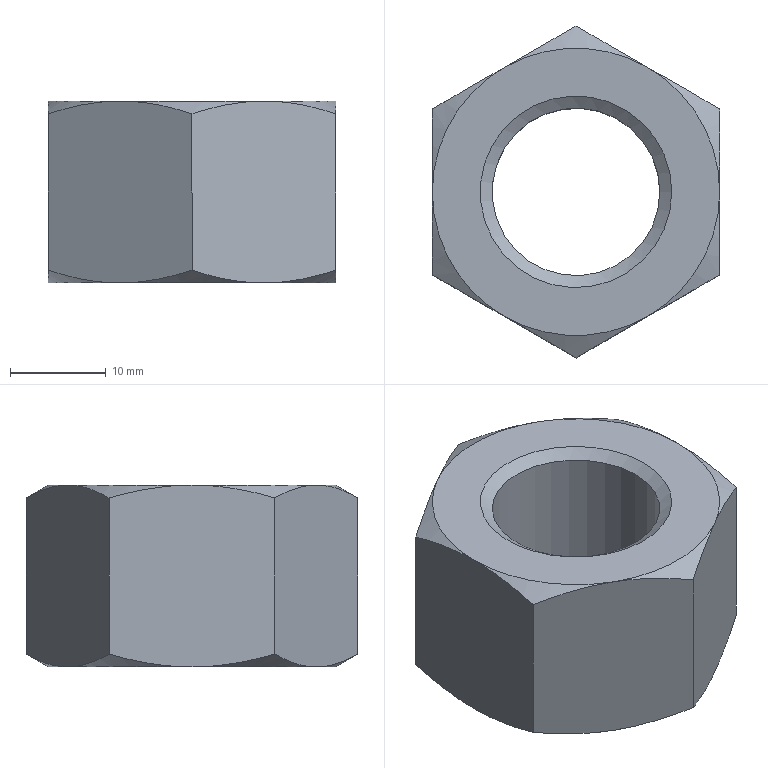Part | NX | features Hexagon Nut ISO - 4034 - M20 - N_Hexagon Nut ISO - 4034 - M20 - N 2 | 1 solid | 24 faces | box 30 x 34.641 x 19 mm | volume 10115 mm3 | cone 14 | plane 8 | cylinder 2 | commonest cylinder face diameters 17.5 x1 20 x1
STEP:
#1=CARTESIAN_POINT('',(7.5,12.99,-19.));
#2=VERTEX_POINT('',#1);
#3=CARTESIAN_POINT('',(15.,8.66,-17.66));
#4=VERTEX_POINT('',#3);
#5=CARTESIAN_POINT('',(7.5,12.99,-19.));
#6=CARTESIAN_POINT('',(10.06,11.512,-19.));
#7=CARTESIAN_POINT('',(12.55,10.075,-18.477));
#8=CARTESIAN_POINT('',(15.,8.66,-17.66));
#9=B_SPLINE_CURVE_WITH_KNOTS('',3,(#5,#6,#7,#8),.UNSPECIFIED.,.F.,.F.,(4,4),(0.,0.008763),.UNSPECIFIED.);
#10=EDGE_CURVE('',#2,#4,#9,.T.);
#11=ORIENTED_EDGE('',*,*,#10,.F.);
#12=CARTESIAN_POINT('',(-0.000000038,17.321,-17.66));
#13=VERTEX_POINT('',#12);
#14=CARTESIAN_POINT('',(-0.000000042,17.321,-17.66));
#15=CARTESIAN_POINT('',(2.45,15.906,-18.477));
#16=CARTESIAN_POINT('',(4.94,14.468,-19.));
#17=CARTESIAN_POINT('',(7.5,12.99,-19.));
#18=B_SPLINE_CURVE_WITH_KNOTS('',3,(#14,#15,#16,#17),.UNSPECIFIED.,.F.,.F.,(4,4),(0.,0.008763),.UNSPECIFIED.);
#19=EDGE_CURVE('',#13,#2,#18,.T.);
#20=ORIENTED_EDGE('',*,*,#19,.F.);
#21=CARTESIAN_POINT('',(0.000000038,17.321,-1.34));
#22=VERTEX_POINT('',#21);
#23=CARTESIAN_POINT('',(0.,17.321,-19.));
#24=DIRECTION('',(0.,0.,1.));
#25=VECTOR('',#24,1000.);
#26=LINE('',#23,#25);
#27=EDGE_CURVE('',#22,#13,#26,.F.);
#28=ORIENTED_EDGE('',*,*,#27,.F.);
#29=CARTESIAN_POINT('',(7.5,12.99,0.));
#30=VERTEX_POINT('',#29);
#31=CARTESIAN_POINT('',(7.5,12.99,0.));
#32=CARTESIAN_POINT('',(4.94,14.468,0.));
#33=CARTESIAN_POINT('',(2.45,15.906,-0.5229));
#34=CARTESIAN_POINT('',(0.000000075,17.321,-1.34));
#35=B_SPLINE_CURVE_WITH_KNOTS('',3,(#31,#32,#33,#34),.UNSPECIFIED.,.F.,.F.,(4,4),(0.,0.008763),.UNSPECIFIED.);
#36=EDGE_CURVE('',#30,#22,#35,.T.);
#37=ORIENTED_EDGE('',*,*,#36,.F.);
#38=CARTESIAN_POINT('',(15.,8.66,-1.34));
#39=VERTEX_POINT('',#38);
#40=CARTESIAN_POINT('',(15.,8.66,-1.34));
#41=CARTESIAN_POINT('',(12.55,10.075,-0.5229));
#42=CARTESIAN_POINT('',(10.06,11.512,0.));
#43=CARTESIAN_POINT('',(7.5,12.99,0.));
#44=B_SPLINE_CURVE_WITH_KNOTS('',3,(#40,#41,#42,#43),.UNSPECIFIED.,.F.,.F.,(4,4),(0.,0.008763),.UNSPECIFIED.);
#45=EDGE_CURVE('',#39,#30,#44,.T.);
#46=ORIENTED_EDGE('',*,*,#45,.F.);
#47=CARTESIAN_POINT('',(15.,8.66,-19.));
#48=DIRECTION('',(0.,0.,1.));
#49=VECTOR('',#48,1000.);
#50=LINE('',#47,#49);
#51=EDGE_CURVE('',#39,#4,#50,.F.);
#52=ORIENTED_EDGE('',*,*,#51,.T.);
#53=EDGE_LOOP('',(#11,#20,#28,#37,#46,#52));
#54=FACE_BOUND('',#53,.T.);
#55=CARTESIAN_POINT('',(15.,8.66,-19.));
#56=DIRECTION('',(0.5,0.866,0.));
#57=DIRECTION('',(-0.866,0.5,0.));
#58=AXIS2_PLACEMENT_3D('',#55,#56,#57);
#59=PLANE('',#58);
#60=ADVANCED_FACE('',(#54),#59,.T.);
#61=CARTESIAN_POINT('',(15.,-8.66,-17.66));
#62=VERTEX_POINT('',#61);
#63=CARTESIAN_POINT('',(15.,-8.66,-1.34));
#64=VERTEX_POINT('',#63);
#65=CARTESIAN_POINT('',(15.,-8.66,-19.));
#66=DIRECTION('',(0.,0.,1.));
#67=VECTOR('',#66,1000.);
#68=LINE('',#65,#67);
#69=EDGE_CURVE('',#62,#64,#68,.T.);
#70=ORIENTED_EDGE('',*,*,#69,.F.);
#71=CARTESIAN_POINT('',(15.,0.,-19.));
#72=VERTEX_POINT('',#71);
#73=CARTESIAN_POINT('',(15.,0.,-19.));
#74=CARTESIAN_POINT('',(15.,-2.956,-19.));
#75=CARTESIAN_POINT('',(15.,-5.831,-18.477));
#76=CARTESIAN_POINT('',(15.,-8.66,-17.66));
#77=B_SPLINE_CURVE_WITH_KNOTS('',3,(#73,#74,#75,#76),.UNSPECIFIED.,.F.,.F.,(4,4),(0.,0.008763),.UNSPECIFIED.);
#78=EDGE_CURVE('',#72,#62,#77,.T.);
#79=ORIENTED_EDGE('',*,*,#78,.F.);
#80=CARTESIAN_POINT('',(15.,8.66,-17.66));
#81=CARTESIAN_POINT('',(15.,5.831,-18.477));
#82=CARTESIAN_POINT('',(15.,2.956,-19.));
#83=CARTESIAN_POINT('',(15.,0.,-19.));
#84=B_SPLINE_CURVE_WITH_KNOTS('',3,(#80,#81,#82,#83),.UNSPECIFIED.,.F.,.F.,(4,4),(0.,0.008763),.UNSPECIFIED.);
#85=EDGE_CURVE('',#4,#72,#84,.T.);
#86=ORIENTED_EDGE('',*,*,#85,.F.);
#87=ORIENTED_EDGE('',*,*,#51,.F.);
#88=CARTESIAN_POINT('',(15.,0.,0.));
#89=VERTEX_POINT('',#88);
#90=CARTESIAN_POINT('',(15.,0.,0.));
#91=CARTESIAN_POINT('',(15.,2.956,0.));
#92=CARTESIAN_POINT('',(15.,5.831,-0.5229));
#93=CARTESIAN_POINT('',(15.,8.66,-1.34));
#94=B_SPLINE_CURVE_WITH_KNOTS('',3,(#90,#91,#92,#93),.UNSPECIFIED.,.F.,.F.,(4,4),(0.,0.008763),.UNSPECIFIED.);
#95=EDGE_CURVE('',#89,#39,#94,.T.);
#96=ORIENTED_EDGE('',*,*,#95,.F.);
#97=CARTESIAN_POINT('',(15.,-8.66,-1.34));
#98=CARTESIAN_POINT('',(15.,-5.831,-0.5229));
#99=CARTESIAN_POINT('',(15.,-2.956,0.));
#100=CARTESIAN_POINT('',(15.,0.,0.));
#101=B_SPLINE_CURVE_WITH_KNOTS('',3,(#97,#98,#99,#100),.UNSPECIFIED.,.F.,.F.,(4,4),(0.,0.008763),.UNSPECIFIED.);
#102=EDGE_CURVE('',#64,#89,#101,.T.);
#103=ORIENTED_EDGE('',*,*,#102,.F.);
#104=EDGE_LOOP('',(#70,#79,#86,#87,#96,#103));
#105=FACE_BOUND('',#104,.T.);
#106=CARTESIAN_POINT('',(15.,8.66,-19.));
#107=DIRECTION('',(-1.,0.,0.));
#108=DIRECTION('',(0.,0.,1.));
#109=AXIS2_PLACEMENT_3D('',#106,#107,#108);
#110=PLANE('',#109);
#111=ADVANCED_FACE('',(#105),#110,.F.);
#112=CARTESIAN_POINT('',(7.5,-12.99,-19.));
#113=VERTEX_POINT('',#112);
#114=CARTESIAN_POINT('',(0.000000038,-17.321,-17.66));
#115=VERTEX_POINT('',#114);
#116=CARTESIAN_POINT('',(7.5,-12.99,-19.));
#117=CARTESIAN_POINT('',(4.94,-14.468,-19.));
#118=CARTESIAN_POINT('',(2.45,-15.906,-18.477));
#119=CARTESIAN_POINT('',(0.000000075,-17.321,-17.66));
#120=B_SPLINE_CURVE_WITH_KNOTS('',3,(#116,#117,#118,#119),.UNSPECIFIED.,.F.,.F.,(4,4),(0.,0.008763),.UNSPECIFIED.);
#121=EDGE_CURVE('',#113,#115,#120,.T.);
#122=ORIENTED_EDGE('',*,*,#121,.F.);
#123=CARTESIAN_POINT('',(15.,-8.66,-17.66));
#124=CARTESIAN_POINT('',(12.55,-10.075,-18.477));
#125=CARTESIAN_POINT('',(10.06,-11.512,-19.));
#126=CARTESIAN_POINT('',(7.5,-12.99,-19.));
#127=B_SPLINE_CURVE_WITH_KNOTS('',3,(#123,#124,#125,#126),.UNSPECIFIED.,.F.,.F.,(4,4),(0.,0.008763),.UNSPECIFIED.);
#128=EDGE_CURVE('',#62,#113,#127,.T.);
#129=ORIENTED_EDGE('',*,*,#128,.F.);
#130=ORIENTED_EDGE('',*,*,#69,.T.);
#131=CARTESIAN_POINT('',(7.5,-12.99,0.));
#132=VERTEX_POINT('',#131);
#133=CARTESIAN_POINT('',(7.5,-12.99,0.));
#134=CARTESIAN_POINT('',(10.06,-11.512,0.));
#135=CARTESIAN_POINT('',(12.55,-10.075,-0.5229));
#136=CARTESIAN_POINT('',(15.,-8.66,-1.34));
#137=B_SPLINE_CURVE_WITH_KNOTS('',3,(#133,#134,#135,#136),.UNSPECIFIED.,.F.,.F.,(4,4),(0.,0.008763),.UNSPECIFIED.);
#138=EDGE_CURVE('',#132,#64,#137,.T.);
#139=ORIENTED_EDGE('',*,*,#138,.F.);
#140=CARTESIAN_POINT('',(-0.000000038,-17.321,-1.34));
#141=VERTEX_POINT('',#140);
#142=CARTESIAN_POINT('',(-0.000000042,-17.321,-1.34));
#143=CARTESIAN_POINT('',(2.45,-15.906,-0.5229));
#144=CARTESIAN_POINT('',(4.94,-14.468,0.));
#145=CARTESIAN_POINT('',(7.5,-12.99,0.));
#146=B_SPLINE_CURVE_WITH_KNOTS('',3,(#142,#143,#144,#145),.UNSPECIFIED.,.F.,.F.,(4,4),(0.,0.008763),.UNSPECIFIED.);
#147=EDGE_CURVE('',#141,#132,#146,.T.);
#148=ORIENTED_EDGE('',*,*,#147,.F.);
#149=CARTESIAN_POINT('',(0.,-17.321,-19.));
#150=DIRECTION('',(0.,0.,1.));
#151=VECTOR('',#150,1000.);
#152=LINE('',#149,#151);
#153=EDGE_CURVE('',#115,#141,#152,.T.);
#154=ORIENTED_EDGE('',*,*,#153,.F.);
#155=EDGE_LOOP('',(#122,#129,#130,#139,#148,#154));
#156=FACE_BOUND('',#155,.T.);
#157=CARTESIAN_POINT('',(0.,-17.321,-19.));
#158=DIRECTION('',(0.5,-0.866,0.));
#159=DIRECTION('',(0.866,0.5,0.));
#160=AXIS2_PLACEMENT_3D('',#157,#158,#159);
#161=PLANE('',#160);
#162=ADVANCED_FACE('',(#156),#161,.T.);
#163=CARTESIAN_POINT('',(-7.5,-12.99,-19.));
#164=VERTEX_POINT('',#163);
#165=CARTESIAN_POINT('',(-15.,-8.66,-17.66));
#166=VERTEX_POINT('',#165);
#167=CARTESIAN_POINT('',(-7.5,-12.99,-19.));
#168=CARTESIAN_POINT('',(-10.06,-11.512,-19.));
#169=CARTESIAN_POINT('',(-12.55,-10.075,-18.477));
#170=CARTESIAN_POINT('',(-15.,-8.66,-17.66));
#171=B_SPLINE_CURVE_WITH_KNOTS('',3,(#167,#168,#169,#170),.UNSPECIFIED.,.F.,.F.,(4,4),(0.,0.008763),.UNSPECIFIED.);
#172=EDGE_CURVE('',#164,#166,#171,.T.);
#173=ORIENTED_EDGE('',*,*,#172,.F.);
#174=CARTESIAN_POINT('',(0.000000042,-17.321,-17.66));
#175=CARTESIAN_POINT('',(-2.45,-15.906,-18.477));
#176=CARTESIAN_POINT('',(-4.94,-14.468,-19.));
#177=CARTESIAN_POINT('',(-7.5,-12.99,-19.));
#178=B_SPLINE_CURVE_WITH_KNOTS('',3,(#174,#175,#176,#177),.UNSPECIFIED.,.F.,.F.,(4,4),(0.,0.008763),.UNSPECIFIED.);
#179=EDGE_CURVE('',#115,#164,#178,.T.);
#180=ORIENTED_EDGE('',*,*,#179,.F.);
#181=ORIENTED_EDGE('',*,*,#153,.T.);
#182=CARTESIAN_POINT('',(-7.5,-12.99,0.));
#183=VERTEX_POINT('',#182);
#184=CARTESIAN_POINT('',(-7.5,-12.99,0.));
#185=CARTESIAN_POINT('',(-4.94,-14.468,0.));
#186=CARTESIAN_POINT('',(-2.45,-15.906,-0.5229));
#187=CARTESIAN_POINT('',(-0.000000075,-17.321,-1.34));
#188=B_SPLINE_CURVE_WITH_KNOTS('',3,(#184,#185,#186,#187),.UNSPECIFIED.,.F.,.F.,(4,4),(0.,0.008763),.UNSPECIFIED.);
#189=EDGE_CURVE('',#183,#141,#188,.T.);
#190=ORIENTED_EDGE('',*,*,#189,.F.);
#191=CARTESIAN_POINT('',(-15.,-8.66,-1.34));
#192=VERTEX_POINT('',#191);
#193=CARTESIAN_POINT('',(-15.,-8.66,-1.34));
#194=CARTESIAN_POINT('',(-12.55,-10.075,-0.5229));
#195=CARTESIAN_POINT('',(-10.06,-11.512,0.));
#196=CARTESIAN_POINT('',(-7.5,-12.99,0.));
#197=B_SPLINE_CURVE_WITH_KNOTS('',3,(#193,#194,#195,#196),.UNSPECIFIED.,.F.,.F.,(4,4),(0.,0.008763),.UNSPECIFIED.);
#198=EDGE_CURVE('',#192,#183,#197,.T.);
#199=ORIENTED_EDGE('',*,*,#198,.F.);
#200=CARTESIAN_POINT('',(-15.,-8.66,-19.));
#201=DIRECTION('',(0.,0.,1.));
#202=VECTOR('',#201,1000.);
#203=LINE('',#200,#202);
#204=EDGE_CURVE('',#166,#192,#203,.T.);
#205=ORIENTED_EDGE('',*,*,#204,.F.);
#206=EDGE_LOOP('',(#173,#180,#181,#190,#199,#205));
#207=FACE_BOUND('',#206,.T.);
#208=CARTESIAN_POINT('',(-15.,-8.66,-19.));
#209=DIRECTION('',(-0.5,-0.866,0.));
#210=DIRECTION('',(0.866,-0.5,0.));
#211=AXIS2_PLACEMENT_3D('',#208,#209,#210);
#212=PLANE('',#211);
#213=ADVANCED_FACE('',(#207),#212,.T.);
#214=CARTESIAN_POINT('',(-15.,0.,-19.));
#215=VERTEX_POINT('',#214);
#216=CARTESIAN_POINT('',(-15.,8.66,-17.66));
#217=VERTEX_POINT('',#216);
#218=CARTESIAN_POINT('',(-15.,0.,-19.));
#219=CARTESIAN_POINT('',(-15.,2.956,-19.));
#220=CARTESIAN_POINT('',(-15.,5.831,-18.477));
#221=CARTESIAN_POINT('',(-15.,8.66,-17.66));
#222=B_SPLINE_CURVE_WITH_KNOTS('',3,(#218,#219,#220,#221),.UNSPECIFIED.,.F.,.F.,(4,4),(0.,0.008763),.UNSPECIFIED.);
#223=EDGE_CURVE('',#215,#217,#222,.T.);
#224=ORIENTED_EDGE('',*,*,#223,.F.);
#225=CARTESIAN_POINT('',(-15.,-8.66,-17.66));
#226=CARTESIAN_POINT('',(-15.,-5.831,-18.477));
#227=CARTESIAN_POINT('',(-15.,-2.956,-19.));
#228=CARTESIAN_POINT('',(-15.,0.,-19.));
#229=B_SPLINE_CURVE_WITH_KNOTS('',3,(#225,#226,#227,#228),.UNSPECIFIED.,.F.,.F.,(4,4),(0.,0.008763),.UNSPECIFIED.);
#230=EDGE_CURVE('',#166,#215,#229,.T.);
#231=ORIENTED_EDGE('',*,*,#230,.F.);
#232=ORIENTED_EDGE('',*,*,#204,.T.);
#233=CARTESIAN_POINT('',(-15.,0.,0.));
#234=VERTEX_POINT('',#233);
#235=CARTESIAN_POINT('',(-15.,0.,0.));
#236=CARTESIAN_POINT('',(-15.,-2.956,0.));
#237=CARTESIAN_POINT('',(-15.,-5.831,-0.5229));
#238=CARTESIAN_POINT('',(-15.,-8.66,-1.34));
#239=B_SPLINE_CURVE_WITH_KNOTS('',3,(#235,#236,#237,#238),.UNSPECIFIED.,.F.,.F.,(4,4),(0.,0.008763),.UNSPECIFIED.);
#240=EDGE_CURVE('',#234,#192,#239,.T.);
#241=ORIENTED_EDGE('',*,*,#240,.F.);
#242=CARTESIAN_POINT('',(-15.,8.66,-1.34));
#243=VERTEX_POINT('',#242);
#244=CARTESIAN_POINT('',(-15.,8.66,-1.34));
#245=CARTESIAN_POINT('',(-15.,5.831,-0.5229));
#246=CARTESIAN_POINT('',(-15.,2.956,0.));
#247=CARTESIAN_POINT('',(-15.,0.,0.));
#248=B_SPLINE_CURVE_WITH_KNOTS('',3,(#244,#245,#246,#247),.UNSPECIFIED.,.F.,.F.,(4,4),(0.,0.008763),.UNSPECIFIED.);
#249=EDGE_CURVE('',#243,#234,#248,.T.);
#250=ORIENTED_EDGE('',*,*,#249,.F.);
#251=CARTESIAN_POINT('',(-15.,8.66,-19.));
#252=DIRECTION('',(0.,0.,1.));
#253=VECTOR('',#252,1000.);
#254=LINE('',#251,#253);
#255=EDGE_CURVE('',#217,#243,#254,.T.);
#256=ORIENTED_EDGE('',*,*,#255,.F.);
#257=EDGE_LOOP('',(#224,#231,#232,#241,#250,#256));
#258=FACE_BOUND('',#257,.T.);
#259=CARTESIAN_POINT('',(-15.,8.66,-19.));
#260=DIRECTION('',(-1.,0.,0.));
#261=DIRECTION('',(0.,0.,1.));
#262=AXIS2_PLACEMENT_3D('',#259,#260,#261);
#263=PLANE('',#262);
#264=ADVANCED_FACE('',(#258),#263,.T.);
#265=CARTESIAN_POINT('',(-7.5,12.99,-19.));
#266=VERTEX_POINT('',#265);
#267=CARTESIAN_POINT('',(-7.5,12.99,-19.));
#268=CARTESIAN_POINT('',(-4.94,14.468,-19.));
#269=CARTESIAN_POINT('',(-2.45,15.906,-18.477));
#270=CARTESIAN_POINT('',(-0.000000075,17.321,-17.66));
#271=B_SPLINE_CURVE_WITH_KNOTS('',3,(#267,#268,#269,#270),.UNSPECIFIED.,.F.,.F.,(4,4),(0.,0.008763),.UNSPECIFIED.);
#272=EDGE_CURVE('',#266,#13,#271,.T.);
#273=ORIENTED_EDGE('',*,*,#272,.F.);
#274=CARTESIAN_POINT('',(-15.,8.66,-17.66));
#275=CARTESIAN_POINT('',(-12.55,10.075,-18.477));
#276=CARTESIAN_POINT('',(-10.06,11.512,-19.));
#277=CARTESIAN_POINT('',(-7.5,12.99,-19.));
#278=B_SPLINE_CURVE_WITH_KNOTS('',3,(#274,#275,#276,#277),.UNSPECIFIED.,.F.,.F.,(4,4),(0.,0.008763),.UNSPECIFIED.);
#279=EDGE_CURVE('',#217,#266,#278,.T.);
#280=ORIENTED_EDGE('',*,*,#279,.F.);
#281=ORIENTED_EDGE('',*,*,#255,.T.);
#282=CARTESIAN_POINT('',(-7.5,12.99,0.));
#283=VERTEX_POINT('',#282);
#284=CARTESIAN_POINT('',(-7.5,12.99,0.));
#285=CARTESIAN_POINT('',(-10.06,11.512,0.));
#286=CARTESIAN_POINT('',(-12.55,10.075,-0.5229));
#287=CARTESIAN_POINT('',(-15.,8.66,-1.34));
#288=B_SPLINE_CURVE_WITH_KNOTS('',3,(#284,#285,#286,#287),.UNSPECIFIED.,.F.,.F.,(4,4),(0.,0.008763),.UNSPECIFIED.);
#289=EDGE_CURVE('',#283,#243,#288,.T.);
#290=ORIENTED_EDGE('',*,*,#289,.F.);
#291=CARTESIAN_POINT('',(0.000000042,17.321,-1.34));
#292=CARTESIAN_POINT('',(-2.45,15.906,-0.5229));
#293=CARTESIAN_POINT('',(-4.94,14.468,0.));
#294=CARTESIAN_POINT('',(-7.5,12.99,0.));
#295=B_SPLINE_CURVE_WITH_KNOTS('',3,(#291,#292,#293,#294),.UNSPECIFIED.,.F.,.F.,(4,4),(0.,0.008763),.UNSPECIFIED.);
#296=EDGE_CURVE('',#22,#283,#295,.T.);
#297=ORIENTED_EDGE('',*,*,#296,.F.);
#298=ORIENTED_EDGE('',*,*,#27,.T.);
#299=EDGE_LOOP('',(#273,#280,#281,#290,#297,#298));
#300=FACE_BOUND('',#299,.T.);
#301=CARTESIAN_POINT('',(0.,17.321,-19.));
#302=DIRECTION('',(-0.5,0.866,0.));
#303=DIRECTION('',(-0.866,-0.5,0.));
#304=AXIS2_PLACEMENT_3D('',#301,#302,#303);
#305=PLANE('',#304);
#306=ADVANCED_FACE('',(#300),#305,.T.);
#307=ORIENTED_EDGE('',*,*,#230,.T.);
#308=CARTESIAN_POINT('',(0.,0.,-19.));
#309=DIRECTION('',(0.,0.,1.));
#310=DIRECTION('',(1.,0.,0.));
#311=AXIS2_PLACEMENT_3D('',#308,#309,#310);
#312=CIRCLE('',#311,15.);
#313=EDGE_CURVE('',#164,#215,#312,.F.);
#314=ORIENTED_EDGE('',*,*,#313,.F.);
#315=ORIENTED_EDGE('',*,*,#172,.T.);
#316=EDGE_LOOP('',(#307,#314,#315));
#317=FACE_BOUND('',#316,.T.);
#318=CARTESIAN_POINT('',(0.,0.,-17.652));
#319=DIRECTION('',(0.,0.,1.));
#320=DIRECTION('',(1.,0.,0.));
#321=AXIS2_PLACEMENT_3D('',#318,#319,#320);
#322=CONICAL_SURFACE('',#321,17.334,1.047);
#323=ADVANCED_FACE('',(#317),#322,.T.);
#324=CARTESIAN_POINT('',(0.,0.,-19.));
#325=DIRECTION('',(0.,0.,1.));
#326=DIRECTION('',(1.,0.,0.));
#327=AXIS2_PLACEMENT_3D('',#324,#325,#326);
#328=CIRCLE('',#327,15.);
#329=EDGE_CURVE('',#215,#266,#328,.F.);
#330=ORIENTED_EDGE('',*,*,#329,.F.);
#331=ORIENTED_EDGE('',*,*,#223,.T.);
#332=ORIENTED_EDGE('',*,*,#279,.T.);
#333=EDGE_LOOP('',(#330,#331,#332));
#334=FACE_BOUND('',#333,.T.);
#335=CARTESIAN_POINT('',(0.,0.,-17.652));
#336=DIRECTION('',(0.,0.,1.));
#337=DIRECTION('',(1.,0.,0.));
#338=AXIS2_PLACEMENT_3D('',#335,#336,#337);
#339=CONICAL_SURFACE('',#338,17.334,1.047);
#340=ADVANCED_FACE('',(#334),#339,.T.);
#341=ORIENTED_EDGE('',*,*,#19,.T.);
#342=CARTESIAN_POINT('',(0.,0.,-19.));
#343=DIRECTION('',(0.,0.,1.));
#344=DIRECTION('',(1.,0.,0.));
#345=AXIS2_PLACEMENT_3D('',#342,#343,#344);
#346=CIRCLE('',#345,15.);
#347=EDGE_CURVE('',#266,#2,#346,.F.);
#348=ORIENTED_EDGE('',*,*,#347,.F.);
#349=ORIENTED_EDGE('',*,*,#272,.T.);
#350=EDGE_LOOP('',(#341,#348,#349));
#351=FACE_BOUND('',#350,.T.);
#352=CARTESIAN_POINT('',(0.,0.,-17.652));
#353=DIRECTION('',(0.,0.,1.));
#354=DIRECTION('',(1.,0.,0.));
#355=AXIS2_PLACEMENT_3D('',#352,#353,#354);
#356=CONICAL_SURFACE('',#355,17.334,1.047);
#357=ADVANCED_FACE('',(#351),#356,.T.);
#358=ORIENTED_EDGE('',*,*,#85,.T.);
#359=CARTESIAN_POINT('',(0.,0.,-19.));
#360=DIRECTION('',(0.,0.,1.));
#361=DIRECTION('',(1.,0.,0.));
#362=AXIS2_PLACEMENT_3D('',#359,#360,#361);
#363=CIRCLE('',#362,15.);
#364=EDGE_CURVE('',#2,#72,#363,.F.);
#365=ORIENTED_EDGE('',*,*,#364,.F.);
#366=ORIENTED_EDGE('',*,*,#10,.T.);
#367=EDGE_LOOP('',(#358,#365,#366));
#368=FACE_BOUND('',#367,.T.);
#369=CARTESIAN_POINT('',(0.,0.,-17.652));
#370=DIRECTION('',(0.,0.,1.));
#371=DIRECTION('',(1.,0.,0.));
#372=AXIS2_PLACEMENT_3D('',#369,#370,#371);
#373=CONICAL_SURFACE('',#372,17.334,1.047);
#374=ADVANCED_FACE('',(#368),#373,.T.);
#375=CARTESIAN_POINT('',(0.,0.,-19.));
#376=DIRECTION('',(0.,0.,1.));
#377=DIRECTION('',(1.,0.,0.));
#378=AXIS2_PLACEMENT_3D('',#375,#376,#377);
#379=CIRCLE('',#378,15.);
#380=EDGE_CURVE('',#72,#113,#379,.F.);
#381=ORIENTED_EDGE('',*,*,#380,.F.);
#382=ORIENTED_EDGE('',*,*,#78,.T.);
#383=ORIENTED_EDGE('',*,*,#128,.T.);
#384=EDGE_LOOP('',(#381,#382,#383));
#385=FACE_BOUND('',#384,.T.);
#386=CARTESIAN_POINT('',(0.,0.,-17.652));
#387=DIRECTION('',(0.,0.,1.));
#388=DIRECTION('',(1.,0.,0.));
#389=AXIS2_PLACEMENT_3D('',#386,#387,#388);
#390=CONICAL_SURFACE('',#389,17.334,1.047);
#391=ADVANCED_FACE('',(#385),#390,.T.);
#392=ORIENTED_EDGE('',*,*,#179,.T.);
#393=CARTESIAN_POINT('',(0.,0.,-19.));
#394=DIRECTION('',(0.,0.,1.));
#395=DIRECTION('',(1.,0.,0.));
#396=AXIS2_PLACEMENT_3D('',#393,#394,#395);
#397=CIRCLE('',#396,15.);
#398=EDGE_CURVE('',#113,#164,#397,.F.);
#399=ORIENTED_EDGE('',*,*,#398,.F.);
#400=ORIENTED_EDGE('',*,*,#121,.T.);
#401=EDGE_LOOP('',(#392,#399,#400));
#402=FACE_BOUND('',#401,.T.);
#403=CARTESIAN_POINT('',(0.,0.,-17.652));
#404=DIRECTION('',(0.,0.,1.));
#405=DIRECTION('',(1.,0.,0.));
#406=AXIS2_PLACEMENT_3D('',#403,#404,#405);
#407=CONICAL_SURFACE('',#406,17.334,1.047);
#408=ADVANCED_FACE('',(#402),#407,.T.);
#409=ORIENTED_EDGE('',*,*,#36,.T.);
#410=ORIENTED_EDGE('',*,*,#296,.T.);
#411=CARTESIAN_POINT('',(0.,0.,0.));
#412=DIRECTION('',(0.,0.,-1.));
#413=DIRECTION('',(-1.,0.,0.));
#414=AXIS2_PLACEMENT_3D('',#411,#412,#413);
#415=CIRCLE('',#414,15.);
#416=EDGE_CURVE('',#283,#30,#415,.T.);
#417=ORIENTED_EDGE('',*,*,#416,.T.);
#418=EDGE_LOOP('',(#409,#410,#417));
#419=FACE_BOUND('',#418,.T.);
#420=CARTESIAN_POINT('',(0.,0.,-1.348));
#421=DIRECTION('',(0.,0.,-1.));
#422=DIRECTION('',(-1.,0.,0.));
#423=AXIS2_PLACEMENT_3D('',#420,#421,#422);
#424=CONICAL_SURFACE('',#423,17.334,1.047);
#425=ADVANCED_FACE('',(#419),#424,.T.);
#426=ORIENTED_EDGE('',*,*,#95,.T.);
#427=ORIENTED_EDGE('',*,*,#45,.T.);
#428=CARTESIAN_POINT('',(0.,0.,0.));
#429=DIRECTION('',(0.,0.,-1.));
#430=DIRECTION('',(-1.,0.,0.));
#431=AXIS2_PLACEMENT_3D('',#428,#429,#430);
#432=CIRCLE('',#431,15.);
#433=EDGE_CURVE('',#30,#89,#432,.T.);
#434=ORIENTED_EDGE('',*,*,#433,.T.);
#435=EDGE_LOOP('',(#426,#427,#434));
#436=FACE_BOUND('',#435,.T.);
#437=CARTESIAN_POINT('',(0.,0.,-1.348));
#438=DIRECTION('',(0.,0.,-1.));
#439=DIRECTION('',(-1.,0.,0.));
#440=AXIS2_PLACEMENT_3D('',#437,#438,#439);
#441=CONICAL_SURFACE('',#440,17.334,1.047);
#442=ADVANCED_FACE('',(#436),#441,.T.);
#443=CARTESIAN_POINT('',(0.,0.,0.));
#444=DIRECTION('',(0.,0.,-1.));
#445=DIRECTION('',(-1.,0.,0.));
#446=AXIS2_PLACEMENT_3D('',#443,#444,#445);
#447=CIRCLE('',#446,15.);
#448=EDGE_CURVE('',#89,#132,#447,.T.);
#449=ORIENTED_EDGE('',*,*,#448,.T.);
#450=ORIENTED_EDGE('',*,*,#138,.T.);
#451=ORIENTED_EDGE('',*,*,#102,.T.);
#452=EDGE_LOOP('',(#449,#450,#451));
#453=FACE_BOUND('',#452,.T.);
#454=CARTESIAN_POINT('',(0.,0.,-1.348));
#455=DIRECTION('',(0.,0.,-1.));
#456=DIRECTION('',(-1.,0.,0.));
#457=AXIS2_PLACEMENT_3D('',#454,#455,#456);
#458=CONICAL_SURFACE('',#457,17.334,1.047);
#459=ADVANCED_FACE('',(#453),#458,.T.);
#460=ORIENTED_EDGE('',*,*,#189,.T.);
#461=ORIENTED_EDGE('',*,*,#147,.T.);
#462=CARTESIAN_POINT('',(0.,0.,0.));
#463=DIRECTION('',(0.,0.,-1.));
#464=DIRECTION('',(-1.,0.,0.));
#465=AXIS2_PLACEMENT_3D('',#462,#463,#464);
#466=CIRCLE('',#465,15.);
#467=EDGE_CURVE('',#132,#183,#466,.T.);
#468=ORIENTED_EDGE('',*,*,#467,.T.);
#469=EDGE_LOOP('',(#460,#461,#468));
#470=FACE_BOUND('',#469,.T.);
#471=CARTESIAN_POINT('',(0.,0.,-1.348));
#472=DIRECTION('',(0.,0.,-1.));
#473=DIRECTION('',(-1.,0.,0.));
#474=AXIS2_PLACEMENT_3D('',#471,#472,#473);
#475=CONICAL_SURFACE('',#474,17.334,1.047);
#476=ADVANCED_FACE('',(#470),#475,.T.);
#477=ORIENTED_EDGE('',*,*,#240,.T.);
#478=ORIENTED_EDGE('',*,*,#198,.T.);
#479=CARTESIAN_POINT('',(0.,0.,0.));
#480=DIRECTION('',(0.,0.,-1.));
#481=DIRECTION('',(-1.,0.,0.));
#482=AXIS2_PLACEMENT_3D('',#479,#480,#481);
#483=CIRCLE('',#482,15.);
#484=EDGE_CURVE('',#183,#234,#483,.T.);
#485=ORIENTED_EDGE('',*,*,#484,.T.);
#486=EDGE_LOOP('',(#477,#478,#485));
#487=FACE_BOUND('',#486,.T.);
#488=CARTESIAN_POINT('',(0.,0.,-1.348));
#489=DIRECTION('',(0.,0.,-1.));
#490=DIRECTION('',(-1.,0.,0.));
#491=AXIS2_PLACEMENT_3D('',#488,#489,#490);
#492=CONICAL_SURFACE('',#491,17.334,1.047);
#493=ADVANCED_FACE('',(#487),#492,.T.);
#494=CARTESIAN_POINT('',(0.,0.,0.));
#495=DIRECTION('',(0.,0.,-1.));
#496=DIRECTION('',(-1.,0.,0.));
#497=AXIS2_PLACEMENT_3D('',#494,#495,#496);
#498=CIRCLE('',#497,15.);
#499=EDGE_CURVE('',#234,#283,#498,.T.);
#500=ORIENTED_EDGE('',*,*,#499,.T.);
#501=ORIENTED_EDGE('',*,*,#289,.T.);
#502=ORIENTED_EDGE('',*,*,#249,.T.);
#503=EDGE_LOOP('',(#500,#501,#502));
#504=FACE_BOUND('',#503,.T.);
#505=CARTESIAN_POINT('',(0.,0.,-1.348));
#506=DIRECTION('',(0.,0.,-1.));
#507=DIRECTION('',(-1.,0.,0.));
#508=AXIS2_PLACEMENT_3D('',#505,#506,#507);
#509=CONICAL_SURFACE('',#508,17.334,1.047);
#510=ADVANCED_FACE('',(#504),#509,.T.);
#511=CARTESIAN_POINT('',(10.,0.,-19.));
#512=VERTEX_POINT('',#511);
#513=CARTESIAN_POINT('',(0.,0.,-19.));
#514=DIRECTION('',(0.,0.,1.));
#515=DIRECTION('',(1.,0.,0.));
#516=AXIS2_PLACEMENT_3D('',#513,#514,#515);
#517=CIRCLE('',#516,10.);
#518=EDGE_CURVE('',#512,#512,#517,.T.);
#519=ORIENTED_EDGE('',*,*,#518,.T.);
#520=EDGE_LOOP('',(#519));
#521=FACE_BOUND('',#520,.T.);
#522=ORIENTED_EDGE('',*,*,#380,.T.);
#523=ORIENTED_EDGE('',*,*,#398,.T.);
#524=ORIENTED_EDGE('',*,*,#313,.T.);
#525=ORIENTED_EDGE('',*,*,#329,.T.);
#526=ORIENTED_EDGE('',*,*,#347,.T.);
#527=ORIENTED_EDGE('',*,*,#364,.T.);
#528=EDGE_LOOP('',(#522,#523,#524,#525,#526,#527));
#529=FACE_BOUND('',#528,.T.);
#530=CARTESIAN_POINT('',(0.,17.321,-19.));
#531=DIRECTION('',(0.,0.,-1.));
#532=DIRECTION('',(-1.,0.,0.));
#533=AXIS2_PLACEMENT_3D('',#530,#531,#532);
#534=PLANE('',#533);
#535=ADVANCED_FACE('',(#521,#529),#534,.T.);
#536=CARTESIAN_POINT('',(10.,0.,0.));
#537=VERTEX_POINT('',#536);
#538=CARTESIAN_POINT('',(0.,0.,0.));
#539=DIRECTION('',(0.,0.,1.));
#540=DIRECTION('',(1.,0.,0.));
#541=AXIS2_PLACEMENT_3D('',#538,#539,#540);
#542=CIRCLE('',#541,10.);
#543=EDGE_CURVE('',#537,#537,#542,.F.);
#544=ORIENTED_EDGE('',*,*,#543,.T.);
#545=EDGE_LOOP('',(#544));
#546=FACE_BOUND('',#545,.T.);
#547=ORIENTED_EDGE('',*,*,#484,.F.);
#548=ORIENTED_EDGE('',*,*,#467,.F.);
#549=ORIENTED_EDGE('',*,*,#448,.F.);
#550=ORIENTED_EDGE('',*,*,#433,.F.);
#551=ORIENTED_EDGE('',*,*,#416,.F.);
#552=ORIENTED_EDGE('',*,*,#499,.F.);
#553=EDGE_LOOP('',(#547,#548,#549,#550,#551,#552));
#554=FACE_BOUND('',#553,.T.);
#555=CARTESIAN_POINT('',(0.,17.321,0.));
#556=DIRECTION('',(0.,0.,-1.));
#557=DIRECTION('',(-1.,0.,0.));
#558=AXIS2_PLACEMENT_3D('',#555,#556,#557);
#559=PLANE('',#558);
#560=ADVANCED_FACE('',(#546,#554),#559,.F.);
#561=ORIENTED_EDGE('',*,*,#518,.F.);
#562=EDGE_LOOP('',(#561));
#563=FACE_BOUND('',#562,.T.);
#564=CARTESIAN_POINT('',(-10.,0.,-18.975));
#565=VERTEX_POINT('',#564);
#566=CARTESIAN_POINT('',(0.,0.,-18.975));
#567=DIRECTION('',(0.,0.,-1.));
#568=DIRECTION('',(-1.,0.,0.));
#569=AXIS2_PLACEMENT_3D('',#566,#567,#568);
#570=CIRCLE('',#569,10.);
#571=EDGE_CURVE('',#565,#565,#570,.F.);
#572=ORIENTED_EDGE('',*,*,#571,.T.);
#573=EDGE_LOOP('',(#572));
#574=FACE_BOUND('',#573,.T.);
#575=CARTESIAN_POINT('',(0.,0.,-25.038));
#576=DIRECTION('',(0.,0.,1.));
#577=DIRECTION('',(1.,0.,0.));
#578=AXIS2_PLACEMENT_3D('',#575,#576,#577);
#579=CYLINDRICAL_SURFACE('',#578,10.);
#580=ADVANCED_FACE('',(#563,#574),#579,.F.);
#581=ORIENTED_EDGE('',*,*,#543,.F.);
#582=EDGE_LOOP('',(#581));
#583=FACE_BOUND('',#582,.T.);
#584=CARTESIAN_POINT('',(8.75,0.,-0.8753));
#585=VERTEX_POINT('',#584);
#586=CARTESIAN_POINT('',(0.,0.,-0.8753));
#587=DIRECTION('',(0.,0.,1.));
#588=DIRECTION('',(1.,0.,0.));
#589=AXIS2_PLACEMENT_3D('',#586,#587,#588);
#590=CIRCLE('',#589,8.75);
#591=EDGE_CURVE('',#585,#585,#590,.F.);
#592=ORIENTED_EDGE('',*,*,#591,.T.);
#593=EDGE_LOOP('',(#592));
#594=FACE_BOUND('',#593,.T.);
#595=CARTESIAN_POINT('',(0.,0.,0.));
#596=DIRECTION('',(0.,0.,1.));
#597=DIRECTION('',(1.,0.,0.));
#598=AXIS2_PLACEMENT_3D('',#595,#596,#597);
#599=CONICAL_SURFACE('',#598,10.,0.9599);
#600=ADVANCED_FACE('',(#583,#594),#599,.F.);
#601=CARTESIAN_POINT('',(8.75,0.,-18.099));
#602=VERTEX_POINT('',#601);
#603=CARTESIAN_POINT('',(0.,0.,-18.099));
#604=DIRECTION('',(0.,0.,1.));
#605=DIRECTION('',(1.,0.,0.));
#606=AXIS2_PLACEMENT_3D('',#603,#604,#605);
#607=CIRCLE('',#606,8.75);
#608=EDGE_CURVE('',#602,#602,#607,.T.);
#609=ORIENTED_EDGE('',*,*,#608,.T.);
#610=EDGE_LOOP('',(#609));
#611=FACE_BOUND('',#610,.T.);
#612=ORIENTED_EDGE('',*,*,#571,.F.);
#613=EDGE_LOOP('',(#612));
#614=FACE_BOUND('',#613,.T.);
#615=CARTESIAN_POINT('',(0.,0.,-18.975));
#616=DIRECTION('',(0.,0.,-1.));
#617=DIRECTION('',(-1.,0.,0.));
#618=AXIS2_PLACEMENT_3D('',#615,#616,#617);
#619=CONICAL_SURFACE('',#618,10.,0.9599);
#620=ADVANCED_FACE('',(#611,#614),#619,.F.);
#621=ORIENTED_EDGE('',*,*,#591,.F.);
#622=EDGE_LOOP('',(#621));
#623=FACE_BOUND('',#622,.T.);
#624=ORIENTED_EDGE('',*,*,#608,.F.);
#625=EDGE_LOOP('',(#624));
#626=FACE_BOUND('',#625,.T.);
#627=CARTESIAN_POINT('',(0.,0.,-19.));
#628=DIRECTION('',(0.,0.,1.));
#629=DIRECTION('',(1.,0.,0.));
#630=AXIS2_PLACEMENT_3D('',#627,#628,#629);
#631=CYLINDRICAL_SURFACE('',#630,8.75);
#632=ADVANCED_FACE('',(#623,#626),#631,.F.);
#633=CLOSED_SHELL('',(#60,#111,#162,#213,#264,#306,#323,#340,#357,#374,#391,#408,#425,#442,#459,#476,#493,#510,#535,#560,#580,#600,#620,#632));
#634=MANIFOLD_SOLID_BREP('',#633);
#635=(LENGTH_UNIT()NAMED_UNIT(*)SI_UNIT(.MILLI.,.METRE.));
#636=UNCERTAINTY_MEASURE_WITH_UNIT(LENGTH_MEASURE(0.0508),#635,'','');
#637=(NAMED_UNIT(*)PLANE_ANGLE_UNIT()SI_UNIT($,.RADIAN.));
#638=(NAMED_UNIT(*)SI_UNIT($,.STERADIAN.)SOLID_ANGLE_UNIT());
#639=(GEOMETRIC_REPRESENTATION_CONTEXT(3)GLOBAL_UNCERTAINTY_ASSIGNED_CONTEXT((#636))GLOBAL_UNIT_ASSIGNED_CONTEXT((#635,#637,#638))REPRESENTATION_CONTEXT('',''));
#640=ADVANCED_BREP_SHAPE_REPRESENTATION('',(#634),#639);